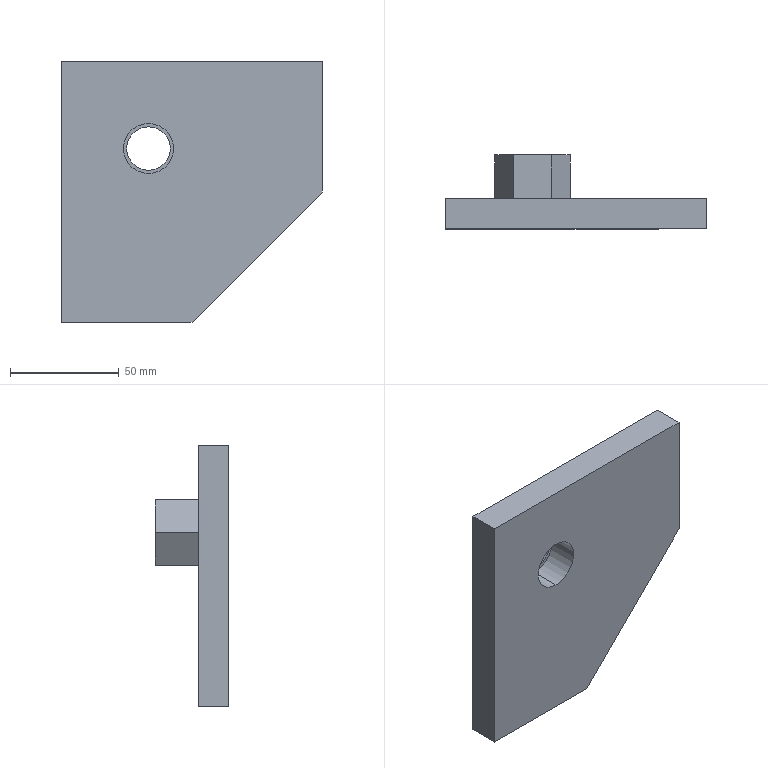Part | SolidWorks | features ICE 2, Extrusion 1 | 1 solid | 19 faces | box 120 x 34 x 120 mm | volume 179889 mm3 | plane 15 | cylinder 4 | commonest cylinder face diameters 20 x2 23 x2
STEP:
#1=CARTESIAN_POINT('',(40.,34.,-50.));
#2=VERTEX_POINT('',#1);
#3=CARTESIAN_POINT('',(40.,34.,-30.));
#4=VERTEX_POINT('',#3);
#5=CARTESIAN_POINT('',(40.,34.,-40.));
#6=DIRECTION('',(0.,1.,0.));
#7=DIRECTION('',(0.,0.,1.));
#8=AXIS2_PLACEMENT_3D('',#5,#6,#7);
#9=CIRCLE('',#8,10.);
#10=EDGE_CURVE('',#2,#4,#9,.T.);
#11=ORIENTED_EDGE('',*,*,#10,.T.);
#12=CARTESIAN_POINT('',(40.,14.,-30.));
#13=VERTEX_POINT('',#12);
#14=CARTESIAN_POINT('',(40.,34.,-30.));
#15=DIRECTION('',(0.,-1.,0.));
#16=VECTOR('',#15,1000.);
#17=LINE('',#14,#16);
#18=EDGE_CURVE('',#4,#13,#17,.T.);
#19=ORIENTED_EDGE('',*,*,#18,.T.);
#20=CARTESIAN_POINT('',(40.,14.,-50.));
#21=VERTEX_POINT('',#20);
#22=CARTESIAN_POINT('',(40.,14.,-40.));
#23=DIRECTION('',(0.,1.,0.));
#24=DIRECTION('',(0.,0.,1.));
#25=AXIS2_PLACEMENT_3D('',#22,#23,#24);
#26=CIRCLE('',#25,10.);
#27=EDGE_CURVE('',#21,#13,#26,.T.);
#28=ORIENTED_EDGE('',*,*,#27,.F.);
#29=CARTESIAN_POINT('',(40.,34.,-50.));
#30=DIRECTION('',(0.,-1.,0.));
#31=VECTOR('',#30,1000.);
#32=LINE('',#29,#31);
#33=EDGE_CURVE('',#2,#21,#32,.T.);
#34=ORIENTED_EDGE('',*,*,#33,.F.);
#35=EDGE_LOOP('',(#11,#19,#28,#34));
#36=FACE_OUTER_BOUND('',#35,.T.);
#37=CARTESIAN_POINT('',(40.,34.,-40.));
#38=DIRECTION('',(0.,-1.,0.));
#39=DIRECTION('',(0.,0.,-1.));
#40=AXIS2_PLACEMENT_3D('',#37,#38,#39);
#41=CYLINDRICAL_SURFACE('',#40,10.);
#42=ADVANCED_FACE('',(#36),#41,.F.);
#43=CARTESIAN_POINT('',(40.,0.,-51.5));
#44=VERTEX_POINT('',#43);
#45=CARTESIAN_POINT('',(40.,0.,-28.5));
#46=VERTEX_POINT('',#45);
#47=CARTESIAN_POINT('',(40.,0.,-40.));
#48=DIRECTION('',(0.,1.,0.));
#49=DIRECTION('',(0.,0.,1.));
#50=AXIS2_PLACEMENT_3D('',#47,#48,#49);
#51=CIRCLE('',#50,11.5);
#52=EDGE_CURVE('',#44,#46,#51,.T.);
#53=ORIENTED_EDGE('',*,*,#52,.F.);
#54=CARTESIAN_POINT('',(40.,14.,-51.5));
#55=VERTEX_POINT('',#54);
#56=CARTESIAN_POINT('',(40.,0.,-51.5));
#57=DIRECTION('',(0.,1.,0.));
#58=VECTOR('',#57,1000.);
#59=LINE('',#56,#58);
#60=EDGE_CURVE('',#44,#55,#59,.T.);
#61=ORIENTED_EDGE('',*,*,#60,.T.);
#62=CARTESIAN_POINT('',(40.,14.,-28.5));
#63=VERTEX_POINT('',#62);
#64=CARTESIAN_POINT('',(40.,14.,-40.));
#65=DIRECTION('',(0.,-1.,0.));
#66=DIRECTION('',(0.,0.,1.));
#67=AXIS2_PLACEMENT_3D('',#64,#65,#66);
#68=CIRCLE('',#67,11.5);
#69=EDGE_CURVE('',#63,#55,#68,.T.);
#70=ORIENTED_EDGE('',*,*,#69,.F.);
#71=CARTESIAN_POINT('',(40.,0.,-28.5));
#72=DIRECTION('',(0.,1.,0.));
#73=VECTOR('',#72,1000.);
#74=LINE('',#71,#73);
#75=EDGE_CURVE('',#46,#63,#74,.T.);
#76=ORIENTED_EDGE('',*,*,#75,.F.);
#77=EDGE_LOOP('',(#53,#61,#70,#76));
#78=FACE_OUTER_BOUND('',#77,.T.);
#79=CARTESIAN_POINT('',(40.,0.,-40.));
#80=DIRECTION('',(0.,1.,0.));
#81=DIRECTION('',(0.,0.,1.));
#82=AXIS2_PLACEMENT_3D('',#79,#80,#81);
#83=CYLINDRICAL_SURFACE('',#82,11.5);
#84=ADVANCED_FACE('',(#78),#83,.F.);
#85=CARTESIAN_POINT('',(0.,14.,0.));
#86=VERTEX_POINT('',#85);
#87=CARTESIAN_POINT('',(120.,14.,0.));
#88=VERTEX_POINT('',#87);
#89=CARTESIAN_POINT('',(120.,14.,0.));
#90=DIRECTION('',(1.,0.,0.));
#91=VECTOR('',#90,1000.);
#92=LINE('',#89,#91);
#93=EDGE_CURVE('',#86,#88,#92,.T.);
#94=ORIENTED_EDGE('',*,*,#93,.T.);
#95=CARTESIAN_POINT('',(120.,14.,-60.));
#96=VERTEX_POINT('',#95);
#97=CARTESIAN_POINT('',(120.,14.,-60.));
#98=DIRECTION('',(0.,0.,-1.));
#99=VECTOR('',#98,1000.);
#100=LINE('',#97,#99);
#101=EDGE_CURVE('',#88,#96,#100,.T.);
#102=ORIENTED_EDGE('',*,*,#101,.T.);
#103=CARTESIAN_POINT('',(60.,14.,-120.));
#104=VERTEX_POINT('',#103);
#105=CARTESIAN_POINT('',(60.,14.,-120.));
#106=DIRECTION('',(-0.7071,0.,-0.7071));
#107=VECTOR('',#106,1000.);
#108=LINE('',#105,#107);
#109=EDGE_CURVE('',#96,#104,#108,.T.);
#110=ORIENTED_EDGE('',*,*,#109,.T.);
#111=CARTESIAN_POINT('',(0.,14.,-120.));
#112=VERTEX_POINT('',#111);
#113=CARTESIAN_POINT('',(0.,14.,-120.));
#114=DIRECTION('',(-1.,0.,0.));
#115=VECTOR('',#114,1000.);
#116=LINE('',#113,#115);
#117=EDGE_CURVE('',#104,#112,#116,.T.);
#118=ORIENTED_EDGE('',*,*,#117,.T.);
#119=CARTESIAN_POINT('',(0.,14.,0.));
#120=DIRECTION('',(0.,0.,1.));
#121=VECTOR('',#120,1000.);
#122=LINE('',#119,#121);
#123=EDGE_CURVE('',#112,#86,#122,.T.);
#124=ORIENTED_EDGE('',*,*,#123,.T.);
#125=EDGE_LOOP('',(#94,#102,#110,#118,#124));
#126=FACE_OUTER_BOUND('',#125,.T.);
#127=CARTESIAN_POINT('',(48.66,14.,-25.));
#128=VERTEX_POINT('',#127);
#129=CARTESIAN_POINT('',(57.321,14.,-40.));
#130=VERTEX_POINT('',#129);
#131=CARTESIAN_POINT('',(48.66,14.,-25.));
#132=DIRECTION('',(0.5,0.,-0.866));
#133=VECTOR('',#132,1000.);
#134=LINE('',#131,#133);
#135=EDGE_CURVE('',#128,#130,#134,.T.);
#136=ORIENTED_EDGE('',*,*,#135,.F.);
#137=CARTESIAN_POINT('',(31.34,14.,-25.));
#138=VERTEX_POINT('',#137);
#139=CARTESIAN_POINT('',(31.34,14.,-25.));
#140=DIRECTION('',(1.,0.,0.));
#141=VECTOR('',#140,1000.);
#142=LINE('',#139,#141);
#143=EDGE_CURVE('',#138,#128,#142,.T.);
#144=ORIENTED_EDGE('',*,*,#143,.F.);
#145=CARTESIAN_POINT('',(22.679,14.,-40.));
#146=VERTEX_POINT('',#145);
#147=CARTESIAN_POINT('',(22.679,14.,-40.));
#148=DIRECTION('',(0.5,0.,0.866));
#149=VECTOR('',#148,1000.);
#150=LINE('',#147,#149);
#151=EDGE_CURVE('',#146,#138,#150,.T.);
#152=ORIENTED_EDGE('',*,*,#151,.F.);
#153=CARTESIAN_POINT('',(31.34,14.,-55.));
#154=VERTEX_POINT('',#153);
#155=CARTESIAN_POINT('',(31.34,14.,-55.));
#156=DIRECTION('',(-0.5,0.,0.866));
#157=VECTOR('',#156,1000.);
#158=LINE('',#155,#157);
#159=EDGE_CURVE('',#154,#146,#158,.T.);
#160=ORIENTED_EDGE('',*,*,#159,.F.);
#161=CARTESIAN_POINT('',(48.66,14.,-55.));
#162=VERTEX_POINT('',#161);
#163=CARTESIAN_POINT('',(48.66,14.,-55.));
#164=DIRECTION('',(-1.,0.,0.));
#165=VECTOR('',#164,1000.);
#166=LINE('',#163,#165);
#167=EDGE_CURVE('',#162,#154,#166,.T.);
#168=ORIENTED_EDGE('',*,*,#167,.F.);
#169=CARTESIAN_POINT('',(57.321,14.,-40.));
#170=DIRECTION('',(-0.5,0.,-0.866));
#171=VECTOR('',#170,1000.);
#172=LINE('',#169,#171);
#173=EDGE_CURVE('',#130,#162,#172,.T.);
#174=ORIENTED_EDGE('',*,*,#173,.F.);
#175=EDGE_LOOP('',(#136,#144,#152,#160,#168,#174));
#176=FACE_BOUND('',#175,.T.);
#177=CARTESIAN_POINT('',(0.,14.,0.));
#178=DIRECTION('',(0.,-1.,0.));
#179=DIRECTION('',(0.,0.,-1.));
#180=AXIS2_PLACEMENT_3D('',#177,#178,#179);
#181=PLANE('',#180);
#182=ADVANCED_FACE('',(#126,#176),#181,.F.);
#183=CARTESIAN_POINT('',(0.,0.,0.));
#184=VERTEX_POINT('',#183);
#185=CARTESIAN_POINT('',(120.,0.,0.));
#186=VERTEX_POINT('',#185);
#187=CARTESIAN_POINT('',(120.,0.,0.));
#188=DIRECTION('',(1.,0.,0.));
#189=VECTOR('',#188,1000.);
#190=LINE('',#187,#189);
#191=EDGE_CURVE('',#184,#186,#190,.T.);
#192=ORIENTED_EDGE('',*,*,#191,.T.);
#193=CARTESIAN_POINT('',(120.,14.,0.));
#194=DIRECTION('',(0.,-1.,0.));
#195=VECTOR('',#194,1000.);
#196=LINE('',#193,#195);
#197=EDGE_CURVE('',#88,#186,#196,.T.);
#198=ORIENTED_EDGE('',*,*,#197,.F.);
#199=ORIENTED_EDGE('',*,*,#93,.F.);
#200=CARTESIAN_POINT('',(0.,14.,0.));
#201=DIRECTION('',(0.,-1.,0.));
#202=VECTOR('',#201,1000.);
#203=LINE('',#200,#202);
#204=EDGE_CURVE('',#86,#184,#203,.T.);
#205=ORIENTED_EDGE('',*,*,#204,.T.);
#206=EDGE_LOOP('',(#192,#198,#199,#205));
#207=FACE_OUTER_BOUND('',#206,.T.);
#208=CARTESIAN_POINT('',(120.,14.,0.));
#209=DIRECTION('',(0.,0.,-1.));
#210=DIRECTION('',(-1.,0.,0.));
#211=AXIS2_PLACEMENT_3D('',#208,#209,#210);
#212=PLANE('',#211);
#213=ADVANCED_FACE('',(#207),#212,.F.);
#214=CARTESIAN_POINT('',(120.,0.,-60.));
#215=VERTEX_POINT('',#214);
#216=CARTESIAN_POINT('',(120.,0.,-60.));
#217=DIRECTION('',(0.,0.,-1.));
#218=VECTOR('',#217,1000.);
#219=LINE('',#216,#218);
#220=EDGE_CURVE('',#186,#215,#219,.T.);
#221=ORIENTED_EDGE('',*,*,#220,.T.);
#222=CARTESIAN_POINT('',(120.,14.,-60.));
#223=DIRECTION('',(0.,-1.,0.));
#224=VECTOR('',#223,1000.);
#225=LINE('',#222,#224);
#226=EDGE_CURVE('',#96,#215,#225,.T.);
#227=ORIENTED_EDGE('',*,*,#226,.F.);
#228=ORIENTED_EDGE('',*,*,#101,.F.);
#229=ORIENTED_EDGE('',*,*,#197,.T.);
#230=EDGE_LOOP('',(#221,#227,#228,#229));
#231=FACE_OUTER_BOUND('',#230,.T.);
#232=CARTESIAN_POINT('',(120.,14.,-60.));
#233=DIRECTION('',(-1.,0.,0.));
#234=DIRECTION('',(0.,0.,1.));
#235=AXIS2_PLACEMENT_3D('',#232,#233,#234);
#236=PLANE('',#235);
#237=ADVANCED_FACE('',(#231),#236,.F.);
#238=CARTESIAN_POINT('',(60.,0.,-120.));
#239=VERTEX_POINT('',#238);
#240=CARTESIAN_POINT('',(60.,0.,-120.));
#241=DIRECTION('',(-0.7071,0.,-0.7071));
#242=VECTOR('',#241,1000.);
#243=LINE('',#240,#242);
#244=EDGE_CURVE('',#215,#239,#243,.T.);
#245=ORIENTED_EDGE('',*,*,#244,.T.);
#246=CARTESIAN_POINT('',(60.,14.,-120.));
#247=DIRECTION('',(0.,-1.,0.));
#248=VECTOR('',#247,1000.);
#249=LINE('',#246,#248);
#250=EDGE_CURVE('',#104,#239,#249,.T.);
#251=ORIENTED_EDGE('',*,*,#250,.F.);
#252=ORIENTED_EDGE('',*,*,#109,.F.);
#253=ORIENTED_EDGE('',*,*,#226,.T.);
#254=EDGE_LOOP('',(#245,#251,#252,#253));
#255=FACE_OUTER_BOUND('',#254,.T.);
#256=CARTESIAN_POINT('',(60.,14.,-120.));
#257=DIRECTION('',(-0.7071,0.,0.7071));
#258=DIRECTION('',(0.7071,0.,0.7071));
#259=AXIS2_PLACEMENT_3D('',#256,#257,#258);
#260=PLANE('',#259);
#261=ADVANCED_FACE('',(#255),#260,.F.);
#262=CARTESIAN_POINT('',(0.,0.,-120.));
#263=VERTEX_POINT('',#262);
#264=CARTESIAN_POINT('',(0.,0.,-120.));
#265=DIRECTION('',(-1.,0.,0.));
#266=VECTOR('',#265,1000.);
#267=LINE('',#264,#266);
#268=EDGE_CURVE('',#239,#263,#267,.T.);
#269=ORIENTED_EDGE('',*,*,#268,.T.);
#270=CARTESIAN_POINT('',(0.,14.,-120.));
#271=DIRECTION('',(0.,-1.,0.));
#272=VECTOR('',#271,1000.);
#273=LINE('',#270,#272);
#274=EDGE_CURVE('',#112,#263,#273,.T.);
#275=ORIENTED_EDGE('',*,*,#274,.F.);
#276=ORIENTED_EDGE('',*,*,#117,.F.);
#277=ORIENTED_EDGE('',*,*,#250,.T.);
#278=EDGE_LOOP('',(#269,#275,#276,#277));
#279=FACE_OUTER_BOUND('',#278,.T.);
#280=CARTESIAN_POINT('',(0.,14.,-120.));
#281=DIRECTION('',(0.,0.,1.));
#282=DIRECTION('',(1.,0.,0.));
#283=AXIS2_PLACEMENT_3D('',#280,#281,#282);
#284=PLANE('',#283);
#285=ADVANCED_FACE('',(#279),#284,.F.);
#286=CARTESIAN_POINT('',(0.,0.,0.));
#287=DIRECTION('',(0.,0.,1.));
#288=VECTOR('',#287,1000.);
#289=LINE('',#286,#288);
#290=EDGE_CURVE('',#263,#184,#289,.T.);
#291=ORIENTED_EDGE('',*,*,#290,.T.);
#292=ORIENTED_EDGE('',*,*,#204,.F.);
#293=ORIENTED_EDGE('',*,*,#123,.F.);
#294=ORIENTED_EDGE('',*,*,#274,.T.);
#295=EDGE_LOOP('',(#291,#292,#293,#294));
#296=FACE_OUTER_BOUND('',#295,.T.);
#297=CARTESIAN_POINT('',(0.,14.,0.));
#298=DIRECTION('',(1.,0.,0.));
#299=DIRECTION('',(0.,0.,-1.));
#300=AXIS2_PLACEMENT_3D('',#297,#298,#299);
#301=PLANE('',#300);
#302=ADVANCED_FACE('',(#296),#301,.F.);
#303=CARTESIAN_POINT('',(40.,0.,-40.));
#304=DIRECTION('',(0.,1.,0.));
#305=DIRECTION('',(0.,0.,1.));
#306=AXIS2_PLACEMENT_3D('',#303,#304,#305);
#307=CIRCLE('',#306,11.5);
#308=EDGE_CURVE('',#46,#44,#307,.T.);
#309=ORIENTED_EDGE('',*,*,#308,.T.);
#310=ORIENTED_EDGE('',*,*,#52,.T.);
#311=EDGE_LOOP('',(#309,#310));
#312=FACE_BOUND('',#311,.T.);
#313=ORIENTED_EDGE('',*,*,#191,.F.);
#314=ORIENTED_EDGE('',*,*,#290,.F.);
#315=ORIENTED_EDGE('',*,*,#268,.F.);
#316=ORIENTED_EDGE('',*,*,#244,.F.);
#317=ORIENTED_EDGE('',*,*,#220,.F.);
#318=EDGE_LOOP('',(#313,#314,#315,#316,#317));
#319=FACE_OUTER_BOUND('',#318,.T.);
#320=CARTESIAN_POINT('',(0.,0.,0.));
#321=DIRECTION('',(0.,-1.,0.));
#322=DIRECTION('',(0.,0.,-1.));
#323=AXIS2_PLACEMENT_3D('',#320,#321,#322);
#324=PLANE('',#323);
#325=ADVANCED_FACE('',(#312,#319),#324,.T.);
#326=ORIENTED_EDGE('',*,*,#60,.F.);
#327=ORIENTED_EDGE('',*,*,#308,.F.);
#328=ORIENTED_EDGE('',*,*,#75,.T.);
#329=CARTESIAN_POINT('',(40.,14.,-40.));
#330=DIRECTION('',(0.,-1.,0.));
#331=DIRECTION('',(0.,0.,1.));
#332=AXIS2_PLACEMENT_3D('',#329,#330,#331);
#333=CIRCLE('',#332,11.5);
#334=EDGE_CURVE('',#55,#63,#333,.T.);
#335=ORIENTED_EDGE('',*,*,#334,.F.);
#336=EDGE_LOOP('',(#326,#327,#328,#335));
#337=FACE_OUTER_BOUND('',#336,.T.);
#338=CARTESIAN_POINT('',(40.,0.,-40.));
#339=DIRECTION('',(0.,1.,0.));
#340=DIRECTION('',(0.,0.,1.));
#341=AXIS2_PLACEMENT_3D('',#338,#339,#340);
#342=CYLINDRICAL_SURFACE('',#341,11.5);
#343=ADVANCED_FACE('',(#337),#342,.F.);
#344=ORIENTED_EDGE('',*,*,#27,.T.);
#345=CARTESIAN_POINT('',(40.,14.,-40.));
#346=DIRECTION('',(0.,1.,0.));
#347=DIRECTION('',(0.,0.,1.));
#348=AXIS2_PLACEMENT_3D('',#345,#346,#347);
#349=CIRCLE('',#348,10.);
#350=EDGE_CURVE('',#13,#21,#349,.T.);
#351=ORIENTED_EDGE('',*,*,#350,.T.);
#352=EDGE_LOOP('',(#344,#351));
#353=FACE_BOUND('',#352,.T.);
#354=ORIENTED_EDGE('',*,*,#69,.T.);
#355=ORIENTED_EDGE('',*,*,#334,.T.);
#356=EDGE_LOOP('',(#354,#355));
#357=FACE_OUTER_BOUND('',#356,.T.);
#358=CARTESIAN_POINT('',(0.,14.,0.));
#359=DIRECTION('',(0.,1.,0.));
#360=DIRECTION('',(0.,0.,1.));
#361=AXIS2_PLACEMENT_3D('',#358,#359,#360);
#362=PLANE('',#361);
#363=ADVANCED_FACE('',(#353,#357),#362,.F.);
#364=CARTESIAN_POINT('',(48.66,34.,-25.));
#365=VERTEX_POINT('',#364);
#366=CARTESIAN_POINT('',(57.321,34.,-40.));
#367=VERTEX_POINT('',#366);
#368=CARTESIAN_POINT('',(48.66,34.,-25.));
#369=DIRECTION('',(0.5,0.,-0.866));
#370=VECTOR('',#369,1000.);
#371=LINE('',#368,#370);
#372=EDGE_CURVE('',#365,#367,#371,.T.);
#373=ORIENTED_EDGE('',*,*,#372,.T.);
#374=CARTESIAN_POINT('',(48.66,34.,-55.));
#375=VERTEX_POINT('',#374);
#376=CARTESIAN_POINT('',(57.321,34.,-40.));
#377=DIRECTION('',(-0.5,0.,-0.866));
#378=VECTOR('',#377,1000.);
#379=LINE('',#376,#378);
#380=EDGE_CURVE('',#367,#375,#379,.T.);
#381=ORIENTED_EDGE('',*,*,#380,.T.);
#382=CARTESIAN_POINT('',(31.34,34.,-55.));
#383=VERTEX_POINT('',#382);
#384=CARTESIAN_POINT('',(48.66,34.,-55.));
#385=DIRECTION('',(-1.,0.,0.));
#386=VECTOR('',#385,1000.);
#387=LINE('',#384,#386);
#388=EDGE_CURVE('',#375,#383,#387,.T.);
#389=ORIENTED_EDGE('',*,*,#388,.T.);
#390=CARTESIAN_POINT('',(22.679,34.,-40.));
#391=VERTEX_POINT('',#390);
#392=CARTESIAN_POINT('',(31.34,34.,-55.));
#393=DIRECTION('',(-0.5,0.,0.866));
#394=VECTOR('',#393,1000.);
#395=LINE('',#392,#394);
#396=EDGE_CURVE('',#383,#391,#395,.T.);
#397=ORIENTED_EDGE('',*,*,#396,.T.);
#398=CARTESIAN_POINT('',(31.34,34.,-25.));
#399=VERTEX_POINT('',#398);
#400=CARTESIAN_POINT('',(22.679,34.,-40.));
#401=DIRECTION('',(0.5,0.,0.866));
#402=VECTOR('',#401,1000.);
#403=LINE('',#400,#402);
#404=EDGE_CURVE('',#391,#399,#403,.T.);
#405=ORIENTED_EDGE('',*,*,#404,.T.);
#406=CARTESIAN_POINT('',(31.34,34.,-25.));
#407=DIRECTION('',(1.,0.,0.));
#408=VECTOR('',#407,1000.);
#409=LINE('',#406,#408);
#410=EDGE_CURVE('',#399,#365,#409,.T.);
#411=ORIENTED_EDGE('',*,*,#410,.T.);
#412=EDGE_LOOP('',(#373,#381,#389,#397,#405,#411));
#413=FACE_OUTER_BOUND('',#412,.T.);
#414=ORIENTED_EDGE('',*,*,#10,.F.);
#415=CARTESIAN_POINT('',(40.,34.,-40.));
#416=DIRECTION('',(0.,1.,0.));
#417=DIRECTION('',(0.,0.,1.));
#418=AXIS2_PLACEMENT_3D('',#415,#416,#417);
#419=CIRCLE('',#418,10.);
#420=EDGE_CURVE('',#4,#2,#419,.T.);
#421=ORIENTED_EDGE('',*,*,#420,.F.);
#422=EDGE_LOOP('',(#414,#421));
#423=FACE_BOUND('',#422,.T.);
#424=CARTESIAN_POINT('',(0.,34.,0.));
#425=DIRECTION('',(0.,1.,0.));
#426=DIRECTION('',(0.,0.,1.));
#427=AXIS2_PLACEMENT_3D('',#424,#425,#426);
#428=PLANE('',#427);
#429=ADVANCED_FACE('',(#413,#423),#428,.T.);
#430=ORIENTED_EDGE('',*,*,#135,.T.);
#431=CARTESIAN_POINT('',(57.321,34.,-40.));
#432=DIRECTION('',(0.,-1.,0.));
#433=VECTOR('',#432,1000.);
#434=LINE('',#431,#433);
#435=EDGE_CURVE('',#367,#130,#434,.T.);
#436=ORIENTED_EDGE('',*,*,#435,.F.);
#437=ORIENTED_EDGE('',*,*,#372,.F.);
#438=CARTESIAN_POINT('',(48.66,34.,-25.));
#439=DIRECTION('',(0.,-1.,0.));
#440=VECTOR('',#439,1000.);
#441=LINE('',#438,#440);
#442=EDGE_CURVE('',#365,#128,#441,.T.);
#443=ORIENTED_EDGE('',*,*,#442,.T.);
#444=EDGE_LOOP('',(#430,#436,#437,#443));
#445=FACE_OUTER_BOUND('',#444,.T.);
#446=CARTESIAN_POINT('',(48.66,34.,-25.));
#447=DIRECTION('',(-0.866,0.,-0.5));
#448=DIRECTION('',(-0.5,0.,0.866));
#449=AXIS2_PLACEMENT_3D('',#446,#447,#448);
#450=PLANE('',#449);
#451=ADVANCED_FACE('',(#445),#450,.F.);
#452=ORIENTED_EDGE('',*,*,#173,.T.);
#453=CARTESIAN_POINT('',(48.66,34.,-55.));
#454=DIRECTION('',(0.,-1.,0.));
#455=VECTOR('',#454,1000.);
#456=LINE('',#453,#455);
#457=EDGE_CURVE('',#375,#162,#456,.T.);
#458=ORIENTED_EDGE('',*,*,#457,.F.);
#459=ORIENTED_EDGE('',*,*,#380,.F.);
#460=ORIENTED_EDGE('',*,*,#435,.T.);
#461=EDGE_LOOP('',(#452,#458,#459,#460));
#462=FACE_OUTER_BOUND('',#461,.T.);
#463=CARTESIAN_POINT('',(57.321,34.,-40.));
#464=DIRECTION('',(-0.866,0.,0.5));
#465=DIRECTION('',(0.5,0.,0.866));
#466=AXIS2_PLACEMENT_3D('',#463,#464,#465);
#467=PLANE('',#466);
#468=ADVANCED_FACE('',(#462),#467,.F.);
#469=ORIENTED_EDGE('',*,*,#167,.T.);
#470=CARTESIAN_POINT('',(31.34,34.,-55.));
#471=DIRECTION('',(0.,-1.,0.));
#472=VECTOR('',#471,1000.);
#473=LINE('',#470,#472);
#474=EDGE_CURVE('',#383,#154,#473,.T.);
#475=ORIENTED_EDGE('',*,*,#474,.F.);
#476=ORIENTED_EDGE('',*,*,#388,.F.);
#477=ORIENTED_EDGE('',*,*,#457,.T.);
#478=EDGE_LOOP('',(#469,#475,#476,#477));
#479=FACE_OUTER_BOUND('',#478,.T.);
#480=CARTESIAN_POINT('',(48.66,34.,-55.));
#481=DIRECTION('',(0.,0.,1.));
#482=DIRECTION('',(1.,0.,0.));
#483=AXIS2_PLACEMENT_3D('',#480,#481,#482);
#484=PLANE('',#483);
#485=ADVANCED_FACE('',(#479),#484,.F.);
#486=ORIENTED_EDGE('',*,*,#159,.T.);
#487=CARTESIAN_POINT('',(22.679,34.,-40.));
#488=DIRECTION('',(0.,-1.,0.));
#489=VECTOR('',#488,1000.);
#490=LINE('',#487,#489);
#491=EDGE_CURVE('',#391,#146,#490,.T.);
#492=ORIENTED_EDGE('',*,*,#491,.F.);
#493=ORIENTED_EDGE('',*,*,#396,.F.);
#494=ORIENTED_EDGE('',*,*,#474,.T.);
#495=EDGE_LOOP('',(#486,#492,#493,#494));
#496=FACE_OUTER_BOUND('',#495,.T.);
#497=CARTESIAN_POINT('',(31.34,34.,-55.));
#498=DIRECTION('',(0.866,0.,0.5));
#499=DIRECTION('',(0.5,0.,-0.866));
#500=AXIS2_PLACEMENT_3D('',#497,#498,#499);
#501=PLANE('',#500);
#502=ADVANCED_FACE('',(#496),#501,.F.);
#503=ORIENTED_EDGE('',*,*,#151,.T.);
#504=CARTESIAN_POINT('',(31.34,34.,-25.));
#505=DIRECTION('',(0.,-1.,0.));
#506=VECTOR('',#505,1000.);
#507=LINE('',#504,#506);
#508=EDGE_CURVE('',#399,#138,#507,.T.);
#509=ORIENTED_EDGE('',*,*,#508,.F.);
#510=ORIENTED_EDGE('',*,*,#404,.F.);
#511=ORIENTED_EDGE('',*,*,#491,.T.);
#512=EDGE_LOOP('',(#503,#509,#510,#511));
#513=FACE_OUTER_BOUND('',#512,.T.);
#514=CARTESIAN_POINT('',(22.679,34.,-40.));
#515=DIRECTION('',(0.866,0.,-0.5));
#516=DIRECTION('',(-0.5,0.,-0.866));
#517=AXIS2_PLACEMENT_3D('',#514,#515,#516);
#518=PLANE('',#517);
#519=ADVANCED_FACE('',(#513),#518,.F.);
#520=ORIENTED_EDGE('',*,*,#143,.T.);
#521=ORIENTED_EDGE('',*,*,#442,.F.);
#522=ORIENTED_EDGE('',*,*,#410,.F.);
#523=ORIENTED_EDGE('',*,*,#508,.T.);
#524=EDGE_LOOP('',(#520,#521,#522,#523));
#525=FACE_OUTER_BOUND('',#524,.T.);
#526=CARTESIAN_POINT('',(31.34,34.,-25.));
#527=DIRECTION('',(0.,0.,-1.));
#528=DIRECTION('',(-1.,0.,0.));
#529=AXIS2_PLACEMENT_3D('',#526,#527,#528);
#530=PLANE('',#529);
#531=ADVANCED_FACE('',(#525),#530,.F.);
#532=ORIENTED_EDGE('',*,*,#18,.F.);
#533=ORIENTED_EDGE('',*,*,#420,.T.);
#534=ORIENTED_EDGE('',*,*,#33,.T.);
#535=ORIENTED_EDGE('',*,*,#350,.F.);
#536=EDGE_LOOP('',(#532,#533,#534,#535));
#537=FACE_OUTER_BOUND('',#536,.T.);
#538=CARTESIAN_POINT('',(40.,34.,-40.));
#539=DIRECTION('',(0.,-1.,0.));
#540=DIRECTION('',(0.,0.,-1.));
#541=AXIS2_PLACEMENT_3D('',#538,#539,#540);
#542=CYLINDRICAL_SURFACE('',#541,10.);
#543=ADVANCED_FACE('',(#537),#542,.F.);
#544=CLOSED_SHELL('',(#42,#84,#182,#213,#237,#261,#285,#302,#325,#343,#363,#429,#451,#468,#485,#502,#519,#531,#543));
#545=MANIFOLD_SOLID_BREP('',#544);
#546=CARTESIAN_POINT('',(0.,0.,0.));
#547=DIRECTION('',(0.,0.,1.));
#548=DIRECTION('',(1.,0.,0.));
#549=AXIS2_PLACEMENT_3D('',#546,#547,#548);
#550=(LENGTH_UNIT()NAMED_UNIT(*)SI_UNIT(.MILLI.,.METRE.));
#551=UNCERTAINTY_MEASURE_WITH_UNIT(LENGTH_MEASURE(0.00001),#550,'','');
#552=(NAMED_UNIT(*)PLANE_ANGLE_UNIT()SI_UNIT($,.RADIAN.));
#553=(NAMED_UNIT(*)SI_UNIT($,.STERADIAN.)SOLID_ANGLE_UNIT());
#554=(GEOMETRIC_REPRESENTATION_CONTEXT(3)GLOBAL_UNCERTAINTY_ASSIGNED_CONTEXT((#551))GLOBAL_UNIT_ASSIGNED_CONTEXT((#550,#552,#553))REPRESENTATION_CONTEXT('',''));
#555=ADVANCED_BREP_SHAPE_REPRESENTATION('',(#545,#549),#554);